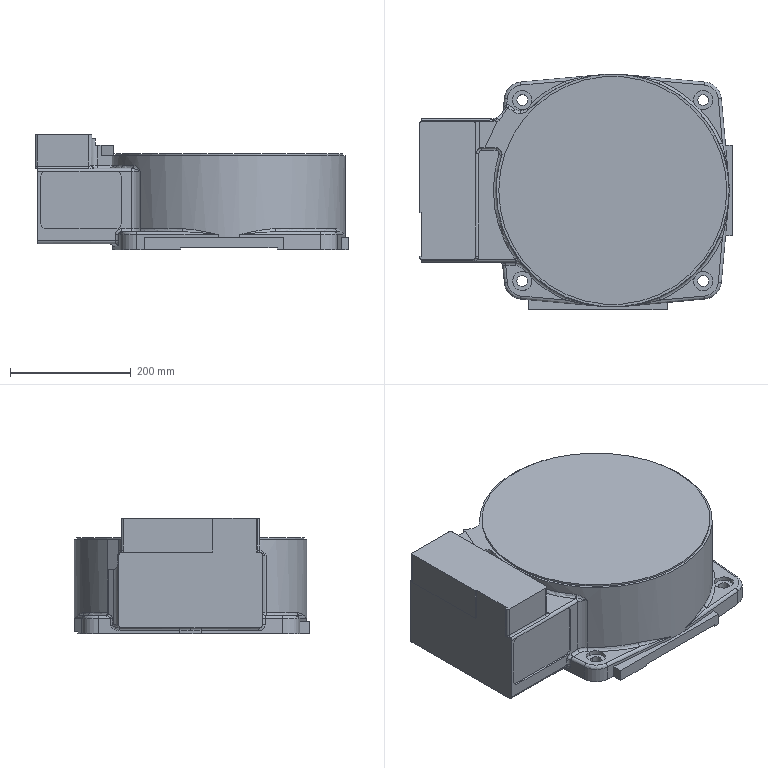Part | STEP file | base | 1 solid | 165 faces | box 518 x 391 x 191.5 mm | volume 24353217 mm3 | cylinder 62 | plane 61 | spline 30 | torus 12 | commonest cylinder face diameters 10 x22 18 x8 32 x8 20 x6 40 x4 60 x4